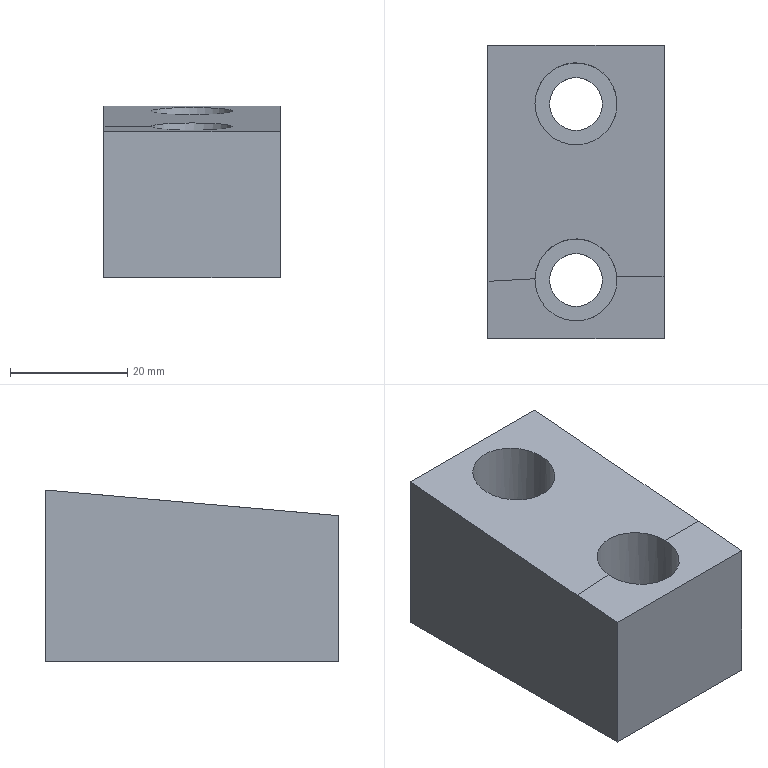Part | NX | features solid 2 | 1 solid | 13 faces | box 30.003 x 50 x 29.308 mm | volume 34139 mm3 | plane 7 | cylinder 4 | spline 2 | commonest cylinder face diameters 9 x2 14 x2
STEP:
#1=CARTESIAN_POINT('',(-512.5,-240.,-69.));
#2=VERTEX_POINT('',#1);
#3=CARTESIAN_POINT('',(-512.5,-240.,-44.066));
#4=VERTEX_POINT('',#3);
#5=CARTESIAN_POINT('',(-512.5,-240.,-74.));
#6=DIRECTION('',(0.,0.,1.));
#7=VECTOR('',#6,1000.);
#8=LINE('',#5,#7);
#9=EDGE_CURVE('',#2,#4,#8,.T.);
#10=ORIENTED_EDGE('',*,*,#9,.T.);
#11=CARTESIAN_POINT('',(-512.5,-230.247,-43.213));
#12=VERTEX_POINT('',#11);
#13=CARTESIAN_POINT('',(-512.5,-192.979,-39.952));
#14=DIRECTION('',(0.,0.9962,0.08716));
#15=VECTOR('',#14,1000.);
#16=LINE('',#13,#15);
#17=EDGE_CURVE('',#4,#12,#16,.T.);
#18=ORIENTED_EDGE('',*,*,#17,.T.);
#19=CARTESIAN_POINT('',(-512.5,-190.,-39.692));
#20=VERTEX_POINT('',#19);
#21=CARTESIAN_POINT('',(-512.5,-192.979,-39.952));
#22=DIRECTION('',(0.,0.9962,0.08716));
#23=VECTOR('',#22,1000.);
#24=LINE('',#21,#23);
#25=EDGE_CURVE('',#20,#12,#24,.F.);
#26=ORIENTED_EDGE('',*,*,#25,.F.);
#27=CARTESIAN_POINT('',(-512.5,-190.,-69.));
#28=VERTEX_POINT('',#27);
#29=CARTESIAN_POINT('',(-512.5,-190.,-74.));
#30=DIRECTION('',(0.,0.,1.));
#31=VECTOR('',#30,1000.);
#32=LINE('',#29,#31);
#33=EDGE_CURVE('',#28,#20,#32,.T.);
#34=ORIENTED_EDGE('',*,*,#33,.F.);
#35=CARTESIAN_POINT('',(-512.5,-190.,-69.));
#36=DIRECTION('',(0.,1.,0.));
#37=VECTOR('',#36,1000.);
#38=LINE('',#35,#37);
#39=EDGE_CURVE('',#28,#2,#38,.F.);
#40=ORIENTED_EDGE('',*,*,#39,.T.);
#41=EDGE_LOOP('',(#10,#18,#26,#34,#40));
#42=FACE_BOUND('',#41,.T.);
#43=CARTESIAN_POINT('',(-512.5,-190.,-74.));
#44=DIRECTION('',(1.,0.,0.));
#45=DIRECTION('',(0.,-1.,0.));
#46=AXIS2_PLACEMENT_3D('',#43,#44,#45);
#47=PLANE('',#46);
#48=ADVANCED_FACE('',(#42),#47,.F.);
#49=CARTESIAN_POINT('',(-482.5,-240.,-69.));
#50=VERTEX_POINT('',#49);
#51=CARTESIAN_POINT('',(-482.5,-240.,-44.066));
#52=VERTEX_POINT('',#51);
#53=CARTESIAN_POINT('',(-482.5,-240.,-74.));
#54=DIRECTION('',(0.,0.,1.));
#55=VECTOR('',#54,1000.);
#56=LINE('',#53,#55);
#57=EDGE_CURVE('',#50,#52,#56,.T.);
#58=ORIENTED_EDGE('',*,*,#57,.T.);
#59=CARTESIAN_POINT('',(-512.5,-240.,-44.066));
#60=DIRECTION('',(-1.,0.,0.));
#61=VECTOR('',#60,1000.);
#62=LINE('',#59,#61);
#63=EDGE_CURVE('',#52,#4,#62,.T.);
#64=ORIENTED_EDGE('',*,*,#63,.T.);
#65=ORIENTED_EDGE('',*,*,#9,.F.);
#66=CARTESIAN_POINT('',(-512.5,-240.,-69.));
#67=DIRECTION('',(-1.,0.,0.));
#68=VECTOR('',#67,1000.);
#69=LINE('',#66,#68);
#70=EDGE_CURVE('',#2,#50,#69,.F.);
#71=ORIENTED_EDGE('',*,*,#70,.T.);
#72=EDGE_LOOP('',(#58,#64,#65,#71));
#73=FACE_BOUND('',#72,.T.);
#74=CARTESIAN_POINT('',(-512.5,-240.,-74.));
#75=DIRECTION('',(0.,1.,0.));
#76=DIRECTION('',(1.,0.,0.));
#77=AXIS2_PLACEMENT_3D('',#74,#75,#76);
#78=PLANE('',#77);
#79=ADVANCED_FACE('',(#73),#78,.F.);
#80=CARTESIAN_POINT('',(-482.5,-229.466,-43.144));
#81=VERTEX_POINT('',#80);
#82=CARTESIAN_POINT('',(-482.5,-190.,-39.692));
#83=VERTEX_POINT('',#82);
#84=CARTESIAN_POINT('',(-482.5,-192.979,-39.952));
#85=DIRECTION('',(0.,0.9962,0.08716));
#86=VECTOR('',#85,1000.);
#87=LINE('',#84,#86);
#88=EDGE_CURVE('',#81,#83,#87,.T.);
#89=ORIENTED_EDGE('',*,*,#88,.F.);
#90=CARTESIAN_POINT('',(-482.5,-192.979,-39.952));
#91=DIRECTION('',(0.,0.9962,0.08716));
#92=VECTOR('',#91,1000.);
#93=LINE('',#90,#92);
#94=EDGE_CURVE('',#81,#52,#93,.F.);
#95=ORIENTED_EDGE('',*,*,#94,.T.);
#96=ORIENTED_EDGE('',*,*,#57,.F.);
#97=CARTESIAN_POINT('',(-482.5,-190.,-69.));
#98=VERTEX_POINT('',#97);
#99=CARTESIAN_POINT('',(-482.5,-190.,-69.));
#100=DIRECTION('',(0.,-1.,0.));
#101=VECTOR('',#100,1000.);
#102=LINE('',#99,#101);
#103=EDGE_CURVE('',#98,#50,#102,.T.);
#104=ORIENTED_EDGE('',*,*,#103,.F.);
#105=CARTESIAN_POINT('',(-482.5,-190.,-74.));
#106=DIRECTION('',(0.,0.,1.));
#107=VECTOR('',#106,1000.);
#108=LINE('',#105,#107);
#109=EDGE_CURVE('',#98,#83,#108,.T.);
#110=ORIENTED_EDGE('',*,*,#109,.T.);
#111=EDGE_LOOP('',(#89,#95,#96,#104,#110));
#112=FACE_BOUND('',#111,.T.);
#113=CARTESIAN_POINT('',(-482.5,-190.,-74.));
#114=DIRECTION('',(1.,0.,0.));
#115=DIRECTION('',(0.,-1.,0.));
#116=AXIS2_PLACEMENT_3D('',#113,#114,#115);
#117=PLANE('',#116);
#118=ADVANCED_FACE('',(#112),#117,.T.);
#119=CARTESIAN_POINT('',(-504.5,-230.,-59.));
#120=VERTEX_POINT('',#119);
#121=CARTESIAN_POINT('',(-497.5,-230.,-59.));
#122=DIRECTION('',(0.,0.,-1.));
#123=DIRECTION('',(-1.,0.,0.));
#124=AXIS2_PLACEMENT_3D('',#121,#122,#123);
#125=CIRCLE('',#124,7.);
#126=EDGE_CURVE('',#120,#120,#125,.T.);
#127=ORIENTED_EDGE('',*,*,#126,.T.);
#128=EDGE_LOOP('',(#127));
#129=FACE_BOUND('',#128,.T.);
#130=CARTESIAN_POINT('',(-490.52,-229.48,-43.146));
#131=VERTEX_POINT('',#130);
#132=CARTESIAN_POINT('',(-504.497,-229.803,-43.174));
#133=VERTEX_POINT('',#132);
#134=CARTESIAN_POINT('',(-490.515,-229.545,-43.151));
#135=CARTESIAN_POINT('',(-490.393,-231.421,-43.316));
#136=CARTESIAN_POINT('',(-491.754,-235.291,-43.654));
#137=CARTESIAN_POINT('',(-497.387,-237.812,-43.875));
#138=CARTESIAN_POINT('',(-503.084,-235.458,-43.669));
#139=CARTESIAN_POINT('',(-504.563,-231.636,-43.334));
#140=CARTESIAN_POINT('',(-504.496,-229.75,-43.169));
#141=B_SPLINE_CURVE_WITH_KNOTS('',3,(#134,#135,#136,#137,#138,#139,#140),.UNSPECIFIED.,.F.,.F.,(4,1,1,1,4),(0.0085,0.01416,0.01982,0.02547,0.03113),.UNSPECIFIED.);
#142=EDGE_CURVE('',#131,#133,#141,.T.);
#143=ORIENTED_EDGE('',*,*,#142,.F.);
#144=CARTESIAN_POINT('',(-490.521,-229.459,-43.144));
#145=CARTESIAN_POINT('',(-490.657,-227.704,-42.99));
#146=CARTESIAN_POINT('',(-492.328,-224.286,-42.691));
#147=CARTESIAN_POINT('',(-497.698,-222.291,-42.517));
#148=CARTESIAN_POINT('',(-502.955,-224.562,-42.715));
#149=CARTESIAN_POINT('',(-504.452,-228.041,-43.02));
#150=CARTESIAN_POINT('',(-504.498,-229.821,-43.175));
#151=B_SPLINE_CURVE_WITH_KNOTS('',3,(#144,#145,#146,#147,#148,#149,#150),.UNSPECIFIED.,.F.,.F.,(4,1,1,1,4),(0.02247,0.02777,0.03307,0.03837,0.04367),.UNSPECIFIED.);
#152=EDGE_CURVE('',#131,#133,#151,.T.);
#153=ORIENTED_EDGE('',*,*,#152,.T.);
#154=EDGE_LOOP('',(#143,#153));
#155=FACE_BOUND('',#154,.T.);
#156=CARTESIAN_POINT('',(-497.5,-230.,26.));
#157=DIRECTION('',(0.,0.,-1.));
#158=DIRECTION('',(-1.,0.,0.));
#159=AXIS2_PLACEMENT_3D('',#156,#157,#158);
#160=CYLINDRICAL_SURFACE('',#159,7.);
#161=ADVANCED_FACE('',(#129,#155),#160,.F.);
#162=CARTESIAN_POINT('',(-512.5,-190.,-39.692));
#163=DIRECTION('',(-1.,0.,0.));
#164=VECTOR('',#163,1000.);
#165=LINE('',#162,#164);
#166=EDGE_CURVE('',#83,#20,#165,.T.);
#167=ORIENTED_EDGE('',*,*,#166,.F.);
#168=ORIENTED_EDGE('',*,*,#109,.F.);
#169=CARTESIAN_POINT('',(-512.5,-190.,-69.));
#170=DIRECTION('',(1.,0.,0.));
#171=VECTOR('',#170,1000.);
#172=LINE('',#169,#171);
#173=EDGE_CURVE('',#28,#98,#172,.T.);
#174=ORIENTED_EDGE('',*,*,#173,.F.);
#175=ORIENTED_EDGE('',*,*,#33,.T.);
#176=EDGE_LOOP('',(#167,#168,#174,#175));
#177=FACE_BOUND('',#176,.T.);
#178=CARTESIAN_POINT('',(-512.5,-190.,-74.));
#179=DIRECTION('',(0.,1.,0.));
#180=DIRECTION('',(1.,0.,0.));
#181=AXIS2_PLACEMENT_3D('',#178,#179,#180);
#182=PLANE('',#181);
#183=ADVANCED_FACE('',(#177),#182,.T.);
#184=CARTESIAN_POINT('',(-502.,-200.,-69.));
#185=VERTEX_POINT('',#184);
#186=CARTESIAN_POINT('',(-497.5,-200.,-69.));
#187=DIRECTION('',(0.,0.,-1.));
#188=DIRECTION('',(-1.,0.,0.));
#189=AXIS2_PLACEMENT_3D('',#186,#187,#188);
#190=CIRCLE('',#189,4.5);
#191=EDGE_CURVE('',#185,#185,#190,.T.);
#192=ORIENTED_EDGE('',*,*,#191,.F.);
#193=EDGE_LOOP('',(#192));
#194=FACE_BOUND('',#193,.T.);
#195=CARTESIAN_POINT('',(-502.,-230.,-69.));
#196=VERTEX_POINT('',#195);
#197=CARTESIAN_POINT('',(-497.5,-230.,-69.));
#198=DIRECTION('',(0.,0.,-1.));
#199=DIRECTION('',(-1.,0.,0.));
#200=AXIS2_PLACEMENT_3D('',#197,#198,#199);
#201=CIRCLE('',#200,4.5);
#202=EDGE_CURVE('',#196,#196,#201,.T.);
#203=ORIENTED_EDGE('',*,*,#202,.F.);
#204=EDGE_LOOP('',(#203));
#205=FACE_BOUND('',#204,.T.);
#206=ORIENTED_EDGE('',*,*,#70,.F.);
#207=ORIENTED_EDGE('',*,*,#39,.F.);
#208=ORIENTED_EDGE('',*,*,#173,.T.);
#209=ORIENTED_EDGE('',*,*,#103,.T.);
#210=EDGE_LOOP('',(#206,#207,#208,#209));
#211=FACE_BOUND('',#210,.T.);
#212=CARTESIAN_POINT('',(-512.5,-190.,-69.));
#213=DIRECTION('',(0.,0.,-1.));
#214=DIRECTION('',(-1.,0.,0.));
#215=AXIS2_PLACEMENT_3D('',#212,#213,#214);
#216=PLANE('',#215);
#217=ADVANCED_FACE('',(#194,#205,#211),#216,.T.);
#218=ORIENTED_EDGE('',*,*,#202,.T.);
#219=EDGE_LOOP('',(#218));
#220=FACE_BOUND('',#219,.T.);
#221=CARTESIAN_POINT('',(-502.,-230.,-59.));
#222=VERTEX_POINT('',#221);
#223=CARTESIAN_POINT('',(-497.5,-230.,-59.));
#224=DIRECTION('',(0.,0.,-1.));
#225=DIRECTION('',(-1.,0.,0.));
#226=AXIS2_PLACEMENT_3D('',#223,#224,#225);
#227=CIRCLE('',#226,4.5);
#228=EDGE_CURVE('',#222,#222,#227,.T.);
#229=ORIENTED_EDGE('',*,*,#228,.F.);
#230=EDGE_LOOP('',(#229));
#231=FACE_BOUND('',#230,.T.);
#232=CARTESIAN_POINT('',(-497.5,-230.,-124.));
#233=DIRECTION('',(0.,0.,-1.));
#234=DIRECTION('',(-1.,0.,0.));
#235=AXIS2_PLACEMENT_3D('',#232,#233,#234);
#236=CYLINDRICAL_SURFACE('',#235,4.5);
#237=ADVANCED_FACE('',(#220,#231),#236,.F.);
#238=ORIENTED_EDGE('',*,*,#228,.T.);
#239=EDGE_LOOP('',(#238));
#240=FACE_BOUND('',#239,.T.);
#241=ORIENTED_EDGE('',*,*,#126,.F.);
#242=EDGE_LOOP('',(#241));
#243=FACE_BOUND('',#242,.T.);
#244=CARTESIAN_POINT('',(-497.5,-230.,-59.));
#245=DIRECTION('',(0.,0.,-1.));
#246=DIRECTION('',(-1.,0.,0.));
#247=AXIS2_PLACEMENT_3D('',#244,#245,#246);
#248=PLANE('',#247);
#249=ADVANCED_FACE('',(#240,#243),#248,.F.);
#250=ORIENTED_EDGE('',*,*,#191,.T.);
#251=EDGE_LOOP('',(#250));
#252=FACE_BOUND('',#251,.T.);
#253=CARTESIAN_POINT('',(-502.,-200.,-59.));
#254=VERTEX_POINT('',#253);
#255=CARTESIAN_POINT('',(-497.5,-200.,-59.));
#256=DIRECTION('',(0.,0.,-1.));
#257=DIRECTION('',(-1.,0.,0.));
#258=AXIS2_PLACEMENT_3D('',#255,#256,#257);
#259=CIRCLE('',#258,4.5);
#260=EDGE_CURVE('',#254,#254,#259,.T.);
#261=ORIENTED_EDGE('',*,*,#260,.F.);
#262=EDGE_LOOP('',(#261));
#263=FACE_BOUND('',#262,.T.);
#264=CARTESIAN_POINT('',(-497.5,-200.,-124.));
#265=DIRECTION('',(0.,0.,-1.));
#266=DIRECTION('',(-1.,0.,0.));
#267=AXIS2_PLACEMENT_3D('',#264,#265,#266);
#268=CYLINDRICAL_SURFACE('',#267,4.5);
#269=ADVANCED_FACE('',(#252,#263),#268,.F.);
#270=ORIENTED_EDGE('',*,*,#260,.T.);
#271=EDGE_LOOP('',(#270));
#272=FACE_BOUND('',#271,.T.);
#273=CARTESIAN_POINT('',(-504.5,-200.,-59.));
#274=VERTEX_POINT('',#273);
#275=CARTESIAN_POINT('',(-497.5,-200.,-59.));
#276=DIRECTION('',(0.,0.,-1.));
#277=DIRECTION('',(-1.,0.,0.));
#278=AXIS2_PLACEMENT_3D('',#275,#276,#277);
#279=CIRCLE('',#278,7.);
#280=EDGE_CURVE('',#274,#274,#279,.T.);
#281=ORIENTED_EDGE('',*,*,#280,.F.);
#282=EDGE_LOOP('',(#281));
#283=FACE_BOUND('',#282,.T.);
#284=CARTESIAN_POINT('',(-497.5,-200.,-59.));
#285=DIRECTION('',(0.,0.,-1.));
#286=DIRECTION('',(-1.,0.,0.));
#287=AXIS2_PLACEMENT_3D('',#284,#285,#286);
#288=PLANE('',#287);
#289=ADVANCED_FACE('',(#272,#283),#288,.F.);
#290=CARTESIAN_POINT('',(-504.5,-200.,-40.566));
#291=VERTEX_POINT('',#290);
#292=CARTESIAN_POINT('',(-502.989,-194.516,-40.087));
#293=CARTESIAN_POINT('',(-505.255,-200.002,-40.567));
#294=CARTESIAN_POINT('',(-502.991,-205.478,-41.046));
#295=CARTESIAN_POINT('',(-497.506,-207.76,-41.245));
#296=CARTESIAN_POINT('',(-492.009,-205.481,-41.046));
#297=CARTESIAN_POINT('',(-489.747,-200.001,-40.567));
#298=CARTESIAN_POINT('',(-492.001,-194.53,-40.088));
#299=CARTESIAN_POINT('',(-497.491,-192.238,-39.887));
#300=CARTESIAN_POINT('',(-502.989,-194.516,-40.087));
#301=CARTESIAN_POINT('',(-505.255,-200.002,-40.567));
#302=CARTESIAN_POINT('',(-502.991,-205.478,-41.046));
#303=B_SPLINE_CURVE_WITH_KNOTS('',3,(#292,#293,#294,#295,#296,#297,#298,#299,#300,#301,#302),.UNSPECIFIED.,.T.,.F.,(1,1,1,1,1,1,1,1,1,1,1,1,1,1,1),(-0.01644,-0.01096,-0.005481,0.,0.005481,0.01096,0.01644,0.02192,0.0274,0.03289,0.03837,0.04385,0.04933,0.05481,0.06029),.UNSPECIFIED.);
#304=EDGE_CURVE('',#291,#291,#303,.T.);
#305=ORIENTED_EDGE('',*,*,#304,.T.);
#306=EDGE_LOOP('',(#305));
#307=FACE_BOUND('',#306,.T.);
#308=ORIENTED_EDGE('',*,*,#280,.T.);
#309=EDGE_LOOP('',(#308));
#310=FACE_BOUND('',#309,.T.);
#311=CARTESIAN_POINT('',(-497.5,-200.,26.));
#312=DIRECTION('',(0.,0.,-1.));
#313=DIRECTION('',(-1.,0.,0.));
#314=AXIS2_PLACEMENT_3D('',#311,#312,#313);
#315=CYLINDRICAL_SURFACE('',#314,7.);
#316=ADVANCED_FACE('',(#307,#310),#315,.F.);
#317=ORIENTED_EDGE('',*,*,#17,.F.);
#318=ORIENTED_EDGE('',*,*,#63,.F.);
#319=ORIENTED_EDGE('',*,*,#94,.F.);
#320=CARTESIAN_POINT('',(-490.518,-229.545,-43.151));
#321=CARTESIAN_POINT('',(-487.846,-229.545,-43.151));
#322=CARTESIAN_POINT('',(-485.173,-229.545,-43.151));
#323=CARTESIAN_POINT('',(-482.5,-229.545,-43.151));
#324=B_SPLINE_CURVE_WITH_KNOTS('',3,(#320,#321,#322,#323),.UNSPECIFIED.,.F.,.F.,(4,4),(0.009219,0.03106),.UNSPECIFIED.);
#325=EDGE_CURVE('',#131,#81,#324,.T.);
#326=ORIENTED_EDGE('',*,*,#325,.F.);
#327=ORIENTED_EDGE('',*,*,#142,.T.);
#328=CARTESIAN_POINT('',(-512.503,-230.178,-43.207));
#329=CARTESIAN_POINT('',(-509.84,-229.996,-43.191));
#330=CARTESIAN_POINT('',(-507.171,-229.853,-43.178));
#331=CARTESIAN_POINT('',(-504.498,-229.75,-43.169));
#332=B_SPLINE_CURVE_WITH_KNOTS('',3,(#328,#329,#330,#331),.UNSPECIFIED.,.F.,.F.,(4,4),(0.9342,0.9626),.UNSPECIFIED.);
#333=EDGE_CURVE('',#12,#133,#332,.T.);
#334=ORIENTED_EDGE('',*,*,#333,.F.);
#335=EDGE_LOOP('',(#317,#318,#319,#326,#327,#334));
#336=FACE_BOUND('',#335,.T.);
#337=CARTESIAN_POINT('',(-512.683,-240.063,-44.072));
#338=CARTESIAN_POINT('',(-482.32,-240.063,-44.072));
#339=CARTESIAN_POINT('',(-512.683,-229.545,-43.151));
#340=CARTESIAN_POINT('',(-482.32,-229.545,-43.151));
#341=B_SPLINE_SURFACE_WITH_KNOTS('',1,1,((#337,#338),(#339,#340)),.PLANE_SURF.,.F.,.F.,.F.,(2,2),(2,2),(0.9336,0.9752),(0.4973,0.5342),.PIECEWISE_BEZIER_KNOTS.);
#342=ADVANCED_FACE('',(#336),#341,.F.);
#343=ORIENTED_EDGE('',*,*,#304,.F.);
#344=EDGE_LOOP('',(#343));
#345=FACE_BOUND('',#344,.T.);
#346=ORIENTED_EDGE('',*,*,#166,.T.);
#347=ORIENTED_EDGE('',*,*,#25,.T.);
#348=ORIENTED_EDGE('',*,*,#333,.T.);
#349=ORIENTED_EDGE('',*,*,#152,.F.);
#350=ORIENTED_EDGE('',*,*,#325,.T.);
#351=ORIENTED_EDGE('',*,*,#88,.T.);
#352=EDGE_LOOP('',(#346,#347,#348,#349,#350,#351));
#353=FACE_BOUND('',#352,.T.);
#354=CARTESIAN_POINT('',(-512.5,-230.512,-43.236));
#355=CARTESIAN_POINT('',(-482.32,-230.512,-43.236));
#356=CARTESIAN_POINT('',(-512.5,-190.,-39.692));
#357=CARTESIAN_POINT('',(-482.32,-190.,-39.692));
#358=B_SPLINE_SURFACE_WITH_KNOTS('',1,1,((#354,#355),(#356,#357)),.PLANE_SURF.,.F.,.F.,.F.,(2,2),(2,2),(0.4514,0.5259),(0.4327,0.4646),.PIECEWISE_BEZIER_KNOTS.);
#359=ADVANCED_FACE('',(#345,#353),#358,.F.);
#360=CLOSED_SHELL('',(#48,#79,#118,#161,#183,#217,#237,#249,#269,#289,#316,#342,#359));
#361=MANIFOLD_SOLID_BREP('',#360);
#362=(LENGTH_UNIT()NAMED_UNIT(*)SI_UNIT(.MILLI.,.METRE.));
#363=UNCERTAINTY_MEASURE_WITH_UNIT(LENGTH_MEASURE(0.2),#362,'','');
#364=(NAMED_UNIT(*)PLANE_ANGLE_UNIT()SI_UNIT($,.RADIAN.));
#365=(NAMED_UNIT(*)SI_UNIT($,.STERADIAN.)SOLID_ANGLE_UNIT());
#366=(GEOMETRIC_REPRESENTATION_CONTEXT(3)GLOBAL_UNCERTAINTY_ASSIGNED_CONTEXT((#363))GLOBAL_UNIT_ASSIGNED_CONTEXT((#362,#364,#365))REPRESENTATION_CONTEXT('',''));
#367=ADVANCED_BREP_SHAPE_REPRESENTATION('',(#361),#366);